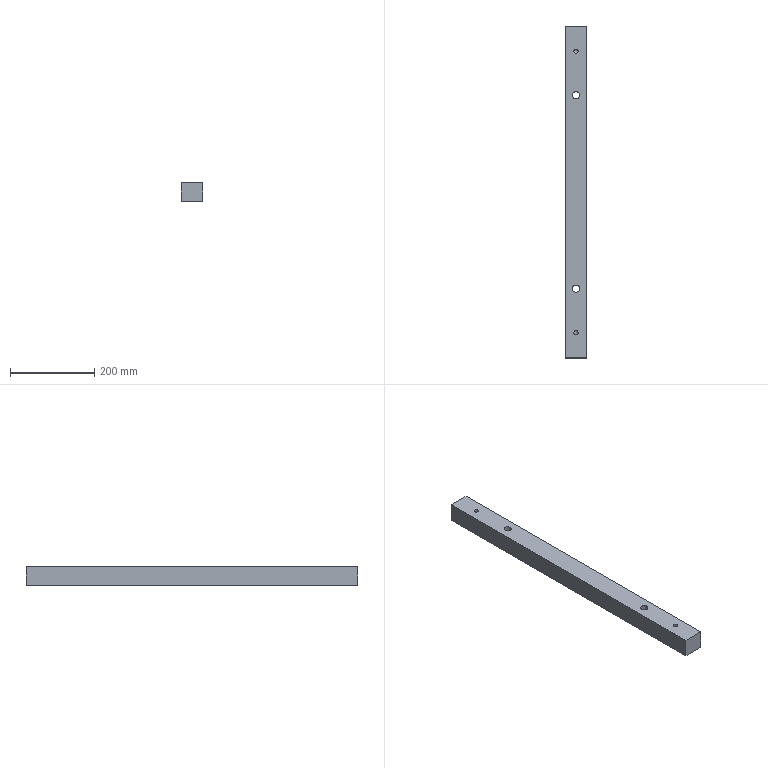Part | STEP file | 020_id2186_x_t | 1 solid | 12 faces | box 50 x 790 x 45 mm | volume 1752403 mm3 | plane 6 | cylinder 4 | cone 2 | commonest cylinder face diameters 10.3 x2 17 x2
STEP:
#1=CARTESIAN_POINT('',(0.,0.,0.));
#2=DIRECTION('',(0.,0.,1.));
#3=DIRECTION('',(1.,0.,0.));
#4=AXIS2_PLACEMENT_3D('',#1,#2,#3);
#5=CARTESIAN_POINT('',(168.35,335.,230.));
#6=VERTEX_POINT('',#5);
#7=CARTESIAN_POINT('',(173.5,335.,230.));
#8=DIRECTION('',(0.,0.,1.));
#9=DIRECTION('',(-1.,0.,0.));
#10=AXIS2_PLACEMENT_3D('',#7,#8,#9);
#11=CIRCLE('',#10,5.15);
#12=CARTESIAN_POINT('',(353.5,-140.,230.));
#13=DIRECTION('',(0.,0.,1.));
#14=DIRECTION('',(1.,0.,0.));
#15=AXIS2_PLACEMENT_3D('',#12,#13,#14);
#16=PLANE('',#15);
#17=CARTESIAN_POINT('',(-180.,475.));
#18=DIRECTION('',(-1.,0.));
#19=AXIS2_PLACEMENT_2D('',#17,#18);
#20=CIRCLE('',#19,5.15);
#21=(GEOMETRIC_REPRESENTATION_CONTEXT(2)PARAMETRIC_REPRESENTATION_CONTEXT()REPRESENTATION_CONTEXT('',''));
#22=DEFINITIONAL_REPRESENTATION('',(#20),#21);
#23=PCURVE('',#16,#22);
#24=CARTESIAN_POINT('',(173.5,335.,259.));
#25=DIRECTION('',(0.,0.,-1.));
#26=DIRECTION('',(-1.,0.,0.));
#27=AXIS2_PLACEMENT_3D('',#24,#25,#26);
#28=CYLINDRICAL_SURFACE('',#27,5.15);
#29=CARTESIAN_POINT('',(6.283,29.));
#30=DIRECTION('',(-1.,0.));
#31=VECTOR('',#30,1.);
#32=LINE('',#29,#31);
#33=(GEOMETRIC_REPRESENTATION_CONTEXT(2)PARAMETRIC_REPRESENTATION_CONTEXT()REPRESENTATION_CONTEXT('',''));
#34=DEFINITIONAL_REPRESENTATION('',(#32),#33);
#35=PCURVE('',#28,#34);
#36=SURFACE_CURVE('',#11,(#23,#35),.PCURVE_S1.);
#37=EDGE_CURVE('',#6,#6,#36,.T.);
#38=ORIENTED_EDGE('',*,*,#37,.F.);
#39=EDGE_LOOP('',(#38));
#40=FACE_BOUND('',#39,.T.);
#41=CARTESIAN_POINT('',(182.,230.,230.));
#42=VERTEX_POINT('',#41);
#43=CARTESIAN_POINT('',(173.5,230.,230.));
#44=DIRECTION('',(0.,0.,-1.));
#45=DIRECTION('',(1.,0.,0.));
#46=AXIS2_PLACEMENT_3D('',#43,#44,#45);
#47=CIRCLE('',#46,8.5);
#48=CARTESIAN_POINT('',(-171.5,370.));
#49=CARTESIAN_POINT('',(-171.5,355.278));
#50=CARTESIAN_POINT('',(-184.25,362.639));
#51=CARTESIAN_POINT('',(-197.,370.));
#52=CARTESIAN_POINT('',(-184.25,377.361));
#53=CARTESIAN_POINT('',(-171.5,384.722));
#54=CARTESIAN_POINT('',(-171.5,370.));
#55=(BOUNDED_CURVE()B_SPLINE_CURVE(2,(#48,#49,#50,#51,#52,#53,#54),.UNSPECIFIED.,.T.,.F.)B_SPLINE_CURVE_WITH_KNOTS((1,2,2,2,2,1),(-2.094,0.,2.094,4.189,6.283,8.378),.UNSPECIFIED.)CURVE()GEOMETRIC_REPRESENTATION_ITEM()RATIONAL_B_SPLINE_CURVE((1.,0.5,1.,0.5,1.,0.5,1.))REPRESENTATION_ITEM(''));
#56=(GEOMETRIC_REPRESENTATION_CONTEXT(2)PARAMETRIC_REPRESENTATION_CONTEXT()REPRESENTATION_CONTEXT('',''));
#57=DEFINITIONAL_REPRESENTATION('',(#55),#56);
#58=PCURVE('',#16,#57);
#59=CARTESIAN_POINT('',(173.5,230.,150.));
#60=DIRECTION('',(0.,0.,1.));
#61=DIRECTION('',(1.,0.,0.));
#62=AXIS2_PLACEMENT_3D('',#59,#60,#61);
#63=CYLINDRICAL_SURFACE('',#62,8.5);
#64=CARTESIAN_POINT('',(6.283,80.));
#65=DIRECTION('',(-1.,0.));
#66=VECTOR('',#65,1.);
#67=LINE('',#64,#66);
#68=(GEOMETRIC_REPRESENTATION_CONTEXT(2)PARAMETRIC_REPRESENTATION_CONTEXT()REPRESENTATION_CONTEXT('',''));
#69=DEFINITIONAL_REPRESENTATION('',(#67),#68);
#70=PCURVE('',#63,#69);
#71=SURFACE_CURVE('',#47,(#58,#70),.PCURVE_S1.);
#72=EDGE_CURVE('',#42,#42,#71,.T.);
#73=ORIENTED_EDGE('',*,*,#72,.T.);
#74=EDGE_LOOP('',(#73));
#75=FACE_BOUND('',#74,.T.);
#76=CARTESIAN_POINT('',(182.,-230.,230.));
#77=VERTEX_POINT('',#76);
#78=CARTESIAN_POINT('',(173.5,-230.,230.));
#79=DIRECTION('',(0.,0.,1.));
#80=DIRECTION('',(1.,0.,0.));
#81=AXIS2_PLACEMENT_3D('',#78,#79,#80);
#82=CIRCLE('',#81,8.5);
#83=CARTESIAN_POINT('',(-180.,-90.));
#84=DIRECTION('',(1.,0.));
#85=AXIS2_PLACEMENT_2D('',#83,#84);
#86=CIRCLE('',#85,8.5);
#87=(GEOMETRIC_REPRESENTATION_CONTEXT(2)PARAMETRIC_REPRESENTATION_CONTEXT()REPRESENTATION_CONTEXT('',''));
#88=DEFINITIONAL_REPRESENTATION('',(#86),#87);
#89=PCURVE('',#16,#88);
#90=CARTESIAN_POINT('',(173.5,-230.,150.));
#91=DIRECTION('',(0.,0.,1.));
#92=DIRECTION('',(1.,0.,0.));
#93=AXIS2_PLACEMENT_3D('',#90,#91,#92);
#94=CYLINDRICAL_SURFACE('',#93,8.5);
#95=CARTESIAN_POINT('',(0.,80.));
#96=DIRECTION('',(1.,0.));
#97=VECTOR('',#96,1.);
#98=LINE('',#95,#97);
#99=(GEOMETRIC_REPRESENTATION_CONTEXT(2)PARAMETRIC_REPRESENTATION_CONTEXT()REPRESENTATION_CONTEXT('',''));
#100=DEFINITIONAL_REPRESENTATION('',(#98),#99);
#101=PCURVE('',#94,#100);
#102=SURFACE_CURVE('',#82,(#89,#101),.PCURVE_S1.);
#103=EDGE_CURVE('',#77,#77,#102,.T.);
#104=ORIENTED_EDGE('',*,*,#103,.F.);
#105=EDGE_LOOP('',(#104));
#106=FACE_BOUND('',#105,.T.);
#107=CARTESIAN_POINT('',(198.5,395.,230.));
#108=VERTEX_POINT('',#107);
#109=CARTESIAN_POINT('',(148.5,395.,230.));
#110=VERTEX_POINT('',#109);
#111=CARTESIAN_POINT('',(353.5,395.,230.));
#112=DIRECTION('',(-1.,0.,0.));
#113=VECTOR('',#112,1.);
#114=LINE('',#111,#113);
#115=CARTESIAN_POINT('',(0.,535.));
#116=DIRECTION('',(-1.,0.));
#117=VECTOR('',#116,1.);
#118=LINE('',#115,#117);
#119=(GEOMETRIC_REPRESENTATION_CONTEXT(2)PARAMETRIC_REPRESENTATION_CONTEXT()REPRESENTATION_CONTEXT('',''));
#120=DEFINITIONAL_REPRESENTATION('',(#118),#119);
#121=PCURVE('',#16,#120);
#122=CARTESIAN_POINT('',(-566.5,395.,-116.5));
#123=DIRECTION('',(0.,1.,0.));
#124=DIRECTION('',(0.,0.,-1.));
#125=AXIS2_PLACEMENT_3D('',#122,#123,#124);
#126=PLANE('',#125);
#127=CARTESIAN_POINT('',(-346.5,-920.));
#128=DIRECTION('',(0.,1.));
#129=VECTOR('',#128,1.);
#130=LINE('',#127,#129);
#131=(GEOMETRIC_REPRESENTATION_CONTEXT(2)PARAMETRIC_REPRESENTATION_CONTEXT()REPRESENTATION_CONTEXT('',''));
#132=DEFINITIONAL_REPRESENTATION('',(#130),#131);
#133=PCURVE('',#126,#132);
#134=SURFACE_CURVE('',#114,(#121,#133),.PCURVE_S1.);
#135=EDGE_CURVE('',#108,#110,#134,.T.);
#136=ORIENTED_EDGE('',*,*,#135,.T.);
#137=CARTESIAN_POINT('',(148.5,-395.,230.));
#138=VERTEX_POINT('',#137);
#139=CARTESIAN_POINT('',(148.5,-350.,230.));
#140=DIRECTION('',(0.,-1.,0.));
#141=VECTOR('',#140,1.);
#142=LINE('',#139,#141);
#143=CARTESIAN_POINT('',(-205.,-210.));
#144=DIRECTION('',(0.,-1.));
#145=VECTOR('',#144,1.);
#146=LINE('',#143,#145);
#147=(GEOMETRIC_REPRESENTATION_CONTEXT(2)PARAMETRIC_REPRESENTATION_CONTEXT()REPRESENTATION_CONTEXT('',''));
#148=DEFINITIONAL_REPRESENTATION('',(#146),#147);
#149=PCURVE('',#16,#148);
#150=CARTESIAN_POINT('',(148.5,-350.,428.5));
#151=DIRECTION('',(-1.,0.,0.));
#152=DIRECTION('',(0.,0.,-1.));
#153=AXIS2_PLACEMENT_3D('',#150,#151,#152);
#154=PLANE('',#153);
#155=CARTESIAN_POINT('',(198.5,0.));
#156=DIRECTION('',(0.,1.));
#157=VECTOR('',#156,1.);
#158=LINE('',#155,#157);
#159=(GEOMETRIC_REPRESENTATION_CONTEXT(2)PARAMETRIC_REPRESENTATION_CONTEXT()REPRESENTATION_CONTEXT('',''));
#160=DEFINITIONAL_REPRESENTATION('',(#158),#159);
#161=PCURVE('',#154,#160);
#162=SURFACE_CURVE('',#142,(#149,#161),.PCURVE_S1.);
#163=EDGE_CURVE('',#110,#138,#162,.T.);
#164=ORIENTED_EDGE('',*,*,#163,.T.);
#165=CARTESIAN_POINT('',(198.5,-395.,230.));
#166=VERTEX_POINT('',#165);
#167=CARTESIAN_POINT('',(353.5,-395.,230.));
#168=DIRECTION('',(-1.,0.,0.));
#169=VECTOR('',#168,1.);
#170=LINE('',#167,#169);
#171=CARTESIAN_POINT('',(0.,-255.));
#172=DIRECTION('',(-1.,0.));
#173=VECTOR('',#172,1.);
#174=LINE('',#171,#173);
#175=(GEOMETRIC_REPRESENTATION_CONTEXT(2)PARAMETRIC_REPRESENTATION_CONTEXT()REPRESENTATION_CONTEXT('',''));
#176=DEFINITIONAL_REPRESENTATION('',(#174),#175);
#177=PCURVE('',#16,#176);
#178=CARTESIAN_POINT('',(-566.5,-395.,-116.5));
#179=DIRECTION('',(0.,-1.,0.));
#180=DIRECTION('',(0.,0.,1.));
#181=AXIS2_PLACEMENT_3D('',#178,#179,#180);
#182=PLANE('',#181);
#183=CARTESIAN_POINT('',(346.5,-920.));
#184=DIRECTION('',(0.,1.));
#185=VECTOR('',#184,1.);
#186=LINE('',#183,#185);
#187=(GEOMETRIC_REPRESENTATION_CONTEXT(2)PARAMETRIC_REPRESENTATION_CONTEXT()REPRESENTATION_CONTEXT('',''));
#188=DEFINITIONAL_REPRESENTATION('',(#186),#187);
#189=PCURVE('',#182,#188);
#190=SURFACE_CURVE('',#170,(#177,#189),.PCURVE_S1.);
#191=EDGE_CURVE('',#166,#138,#190,.T.);
#192=ORIENTED_EDGE('',*,*,#191,.F.);
#193=CARTESIAN_POINT('',(198.5,-350.,230.));
#194=DIRECTION('',(0.,1.,0.));
#195=VECTOR('',#194,1.);
#196=LINE('',#193,#195);
#197=CARTESIAN_POINT('',(-155.,-210.));
#198=DIRECTION('',(0.,1.));
#199=VECTOR('',#198,1.);
#200=LINE('',#197,#199);
#201=(GEOMETRIC_REPRESENTATION_CONTEXT(2)PARAMETRIC_REPRESENTATION_CONTEXT()REPRESENTATION_CONTEXT('',''));
#202=DEFINITIONAL_REPRESENTATION('',(#200),#201);
#203=PCURVE('',#16,#202);
#204=CARTESIAN_POINT('',(198.5,-350.,428.5));
#205=DIRECTION('',(-1.,0.,0.));
#206=DIRECTION('',(0.,0.,-1.));
#207=AXIS2_PLACEMENT_3D('',#204,#205,#206);
#208=PLANE('',#207);
#209=CARTESIAN_POINT('',(198.5,0.));
#210=DIRECTION('',(0.,-1.));
#211=VECTOR('',#210,1.);
#212=LINE('',#209,#211);
#213=(GEOMETRIC_REPRESENTATION_CONTEXT(2)PARAMETRIC_REPRESENTATION_CONTEXT()REPRESENTATION_CONTEXT('',''));
#214=DEFINITIONAL_REPRESENTATION('',(#212),#213);
#215=PCURVE('',#208,#214);
#216=SURFACE_CURVE('',#196,(#203,#215),.PCURVE_S1.);
#217=EDGE_CURVE('',#166,#108,#216,.T.);
#218=ORIENTED_EDGE('',*,*,#217,.T.);
#219=EDGE_LOOP('',(#136,#164,#192,#218));
#220=FACE_BOUND('',#219,.T.);
#221=CARTESIAN_POINT('',(168.35,-335.,230.));
#222=VERTEX_POINT('',#221);
#223=CARTESIAN_POINT('',(173.5,-335.,230.));
#224=DIRECTION('',(0.,0.,-1.));
#225=DIRECTION('',(-1.,0.,0.));
#226=AXIS2_PLACEMENT_3D('',#223,#224,#225);
#227=CIRCLE('',#226,5.15);
#228=CARTESIAN_POINT('',(-185.15,-195.));
#229=CARTESIAN_POINT('',(-185.15,-186.08));
#230=CARTESIAN_POINT('',(-177.425,-190.54));
#231=CARTESIAN_POINT('',(-169.7,-195.));
#232=CARTESIAN_POINT('',(-177.425,-199.46));
#233=CARTESIAN_POINT('',(-185.15,-203.92));
#234=CARTESIAN_POINT('',(-185.15,-195.));
#235=(BOUNDED_CURVE()B_SPLINE_CURVE(2,(#228,#229,#230,#231,#232,#233,#234),.UNSPECIFIED.,.T.,.F.)B_SPLINE_CURVE_WITH_KNOTS((1,2,2,2,2,1),(-2.094,0.,2.094,4.189,6.283,8.378),.UNSPECIFIED.)CURVE()GEOMETRIC_REPRESENTATION_ITEM()RATIONAL_B_SPLINE_CURVE((1.,0.5,1.,0.5,1.,0.5,1.))REPRESENTATION_ITEM(''));
#236=(GEOMETRIC_REPRESENTATION_CONTEXT(2)PARAMETRIC_REPRESENTATION_CONTEXT()REPRESENTATION_CONTEXT('',''));
#237=DEFINITIONAL_REPRESENTATION('',(#235),#236);
#238=PCURVE('',#16,#237);
#239=CARTESIAN_POINT('',(173.5,-335.,259.));
#240=DIRECTION('',(0.,0.,-1.));
#241=DIRECTION('',(-1.,0.,0.));
#242=AXIS2_PLACEMENT_3D('',#239,#240,#241);
#243=CYLINDRICAL_SURFACE('',#242,5.15);
#244=CARTESIAN_POINT('',(0.,29.));
#245=DIRECTION('',(1.,0.));
#246=VECTOR('',#245,1.);
#247=LINE('',#244,#246);
#248=(GEOMETRIC_REPRESENTATION_CONTEXT(2)PARAMETRIC_REPRESENTATION_CONTEXT()REPRESENTATION_CONTEXT('',''));
#249=DEFINITIONAL_REPRESENTATION('',(#247),#248);
#250=PCURVE('',#243,#249);
#251=SURFACE_CURVE('',#227,(#238,#250),.PCURVE_S1.);
#252=EDGE_CURVE('',#222,#222,#251,.T.);
#253=ORIENTED_EDGE('',*,*,#252,.T.);
#254=EDGE_LOOP('',(#253));
#255=FACE_BOUND('',#254,.T.);
#256=ADVANCED_FACE('',(#40,#75,#106,#220,#255),#16,.T.);
#257=CARTESIAN_POINT('',(198.5,-395.,185.));
#258=VERTEX_POINT('',#257);
#259=CARTESIAN_POINT('',(148.5,-395.,185.));
#260=VERTEX_POINT('',#259);
#261=CARTESIAN_POINT('',(-566.5,-395.,185.));
#262=DIRECTION('',(-1.,0.,0.));
#263=VECTOR('',#262,1.);
#264=LINE('',#261,#263);
#265=CARTESIAN_POINT('',(148.5,-350.,185.));
#266=DIRECTION('',(0.,0.,1.));
#267=DIRECTION('',(0.,-1.,0.));
#268=AXIS2_PLACEMENT_3D('',#265,#266,#267);
#269=PLANE('',#268);
#270=CARTESIAN_POINT('',(45.,-715.));
#271=DIRECTION('',(0.,-1.));
#272=VECTOR('',#271,1.);
#273=LINE('',#270,#272);
#274=(GEOMETRIC_REPRESENTATION_CONTEXT(2)PARAMETRIC_REPRESENTATION_CONTEXT()REPRESENTATION_CONTEXT('',''));
#275=DEFINITIONAL_REPRESENTATION('',(#273),#274);
#276=PCURVE('',#269,#275);
#277=CARTESIAN_POINT('',(301.5,0.));
#278=DIRECTION('',(0.,1.));
#279=VECTOR('',#278,1.);
#280=LINE('',#277,#279);
#281=(GEOMETRIC_REPRESENTATION_CONTEXT(2)PARAMETRIC_REPRESENTATION_CONTEXT()REPRESENTATION_CONTEXT('',''));
#282=DEFINITIONAL_REPRESENTATION('',(#280),#281);
#283=PCURVE('',#182,#282);
#284=SURFACE_CURVE('',#264,(#276,#283),.PCURVE_S1.);
#285=EDGE_CURVE('',#258,#260,#284,.T.);
#286=ORIENTED_EDGE('',*,*,#285,.T.);
#287=CARTESIAN_POINT('',(148.5,395.,185.));
#288=VERTEX_POINT('',#287);
#289=CARTESIAN_POINT('',(148.5,-350.,185.));
#290=DIRECTION('',(0.,1.,0.));
#291=VECTOR('',#290,1.);
#292=LINE('',#289,#291);
#293=CARTESIAN_POINT('',(0.,0.));
#294=DIRECTION('',(-1.,0.));
#295=VECTOR('',#294,1.);
#296=LINE('',#293,#295);
#297=(GEOMETRIC_REPRESENTATION_CONTEXT(2)PARAMETRIC_REPRESENTATION_CONTEXT()REPRESENTATION_CONTEXT('',''));
#298=DEFINITIONAL_REPRESENTATION('',(#296),#297);
#299=PCURVE('',#269,#298);
#300=CARTESIAN_POINT('',(243.5,0.));
#301=DIRECTION('',(0.,-1.));
#302=VECTOR('',#301,1.);
#303=LINE('',#300,#302);
#304=(GEOMETRIC_REPRESENTATION_CONTEXT(2)PARAMETRIC_REPRESENTATION_CONTEXT()REPRESENTATION_CONTEXT('',''));
#305=DEFINITIONAL_REPRESENTATION('',(#303),#304);
#306=PCURVE('',#154,#305);
#307=SURFACE_CURVE('',#292,(#299,#306),.PCURVE_S1.);
#308=EDGE_CURVE('',#260,#288,#307,.T.);
#309=ORIENTED_EDGE('',*,*,#308,.T.);
#310=CARTESIAN_POINT('',(198.5,395.,185.));
#311=VERTEX_POINT('',#310);
#312=CARTESIAN_POINT('',(148.5,395.,185.));
#313=DIRECTION('',(-1.,0.,0.));
#314=VECTOR('',#313,1.);
#315=LINE('',#312,#314);
#316=CARTESIAN_POINT('',(-745.,0.));
#317=DIRECTION('',(0.,-1.));
#318=VECTOR('',#317,1.);
#319=LINE('',#316,#318);
#320=(GEOMETRIC_REPRESENTATION_CONTEXT(2)PARAMETRIC_REPRESENTATION_CONTEXT()REPRESENTATION_CONTEXT('',''));
#321=DEFINITIONAL_REPRESENTATION('',(#319),#320);
#322=PCURVE('',#269,#321);
#323=CARTESIAN_POINT('',(-301.5,-715.));
#324=DIRECTION('',(0.,1.));
#325=VECTOR('',#324,1.);
#326=LINE('',#323,#325);
#327=(GEOMETRIC_REPRESENTATION_CONTEXT(2)PARAMETRIC_REPRESENTATION_CONTEXT()REPRESENTATION_CONTEXT('',''));
#328=DEFINITIONAL_REPRESENTATION('',(#326),#327);
#329=PCURVE('',#126,#328);
#330=SURFACE_CURVE('',#315,(#322,#329),.PCURVE_S1.);
#331=EDGE_CURVE('',#311,#288,#330,.T.);
#332=ORIENTED_EDGE('',*,*,#331,.F.);
#333=CARTESIAN_POINT('',(198.5,-350.,185.));
#334=DIRECTION('',(0.,1.,0.));
#335=VECTOR('',#334,1.);
#336=LINE('',#333,#335);
#337=CARTESIAN_POINT('',(0.,50.));
#338=DIRECTION('',(-1.,0.));
#339=VECTOR('',#338,1.);
#340=LINE('',#337,#339);
#341=(GEOMETRIC_REPRESENTATION_CONTEXT(2)PARAMETRIC_REPRESENTATION_CONTEXT()REPRESENTATION_CONTEXT('',''));
#342=DEFINITIONAL_REPRESENTATION('',(#340),#341);
#343=PCURVE('',#269,#342);
#344=CARTESIAN_POINT('',(243.5,0.));
#345=DIRECTION('',(0.,-1.));
#346=VECTOR('',#345,1.);
#347=LINE('',#344,#346);
#348=(GEOMETRIC_REPRESENTATION_CONTEXT(2)PARAMETRIC_REPRESENTATION_CONTEXT()REPRESENTATION_CONTEXT('',''));
#349=DEFINITIONAL_REPRESENTATION('',(#347),#348);
#350=PCURVE('',#208,#349);
#351=SURFACE_CURVE('',#336,(#343,#350),.PCURVE_S1.);
#352=EDGE_CURVE('',#258,#311,#351,.T.);
#353=ORIENTED_EDGE('',*,*,#352,.F.);
#354=EDGE_LOOP('',(#286,#309,#332,#353));
#355=FACE_BOUND('',#354,.T.);
#356=CARTESIAN_POINT('',(182.,-230.,185.));
#357=VERTEX_POINT('',#356);
#358=CARTESIAN_POINT('',(173.5,-230.,185.));
#359=DIRECTION('',(0.,0.,1.));
#360=DIRECTION('',(1.,0.,0.));
#361=AXIS2_PLACEMENT_3D('',#358,#359,#360);
#362=CIRCLE('',#361,8.5);
#363=CARTESIAN_POINT('',(-120.,25.));
#364=DIRECTION('',(0.,1.));
#365=AXIS2_PLACEMENT_2D('',#363,#364);
#366=CIRCLE('',#365,8.5);
#367=(GEOMETRIC_REPRESENTATION_CONTEXT(2)PARAMETRIC_REPRESENTATION_CONTEXT()REPRESENTATION_CONTEXT('',''));
#368=DEFINITIONAL_REPRESENTATION('',(#366),#367);
#369=PCURVE('',#269,#368);
#370=CARTESIAN_POINT('',(0.,35.));
#371=DIRECTION('',(1.,0.));
#372=VECTOR('',#371,1.);
#373=LINE('',#370,#372);
#374=(GEOMETRIC_REPRESENTATION_CONTEXT(2)PARAMETRIC_REPRESENTATION_CONTEXT()REPRESENTATION_CONTEXT('',''));
#375=DEFINITIONAL_REPRESENTATION('',(#373),#374);
#376=PCURVE('',#94,#375);
#377=SURFACE_CURVE('',#362,(#369,#376),.PCURVE_S1.);
#378=EDGE_CURVE('',#357,#357,#377,.T.);
#379=ORIENTED_EDGE('',*,*,#378,.T.);
#380=EDGE_LOOP('',(#379));
#381=FACE_BOUND('',#380,.T.);
#382=CARTESIAN_POINT('',(182.,230.,185.));
#383=VERTEX_POINT('',#382);
#384=CARTESIAN_POINT('',(173.5,230.,185.));
#385=DIRECTION('',(0.,0.,-1.));
#386=DIRECTION('',(1.,0.,0.));
#387=AXIS2_PLACEMENT_3D('',#384,#385,#386);
#388=CIRCLE('',#387,8.5);
#389=CARTESIAN_POINT('',(-580.,33.5));
#390=CARTESIAN_POINT('',(-565.278,33.5));
#391=CARTESIAN_POINT('',(-572.639,20.75));
#392=CARTESIAN_POINT('',(-580.,8.));
#393=CARTESIAN_POINT('',(-587.361,20.75));
#394=CARTESIAN_POINT('',(-594.722,33.5));
#395=CARTESIAN_POINT('',(-580.,33.5));
#396=(BOUNDED_CURVE()B_SPLINE_CURVE(2,(#389,#390,#391,#392,#393,#394,#395),.UNSPECIFIED.,.T.,.F.)B_SPLINE_CURVE_WITH_KNOTS((1,2,2,2,2,1),(-2.094,0.,2.094,4.189,6.283,8.378),.UNSPECIFIED.)CURVE()GEOMETRIC_REPRESENTATION_ITEM()RATIONAL_B_SPLINE_CURVE((1.,0.5,1.,0.5,1.,0.5,1.))REPRESENTATION_ITEM(''));
#397=(GEOMETRIC_REPRESENTATION_CONTEXT(2)PARAMETRIC_REPRESENTATION_CONTEXT()REPRESENTATION_CONTEXT('',''));
#398=DEFINITIONAL_REPRESENTATION('',(#396),#397);
#399=PCURVE('',#269,#398);
#400=CARTESIAN_POINT('',(6.283,35.));
#401=DIRECTION('',(-1.,0.));
#402=VECTOR('',#401,1.);
#403=LINE('',#400,#402);
#404=(GEOMETRIC_REPRESENTATION_CONTEXT(2)PARAMETRIC_REPRESENTATION_CONTEXT()REPRESENTATION_CONTEXT('',''));
#405=DEFINITIONAL_REPRESENTATION('',(#403),#404);
#406=PCURVE('',#63,#405);
#407=SURFACE_CURVE('',#388,(#399,#406),.PCURVE_S1.);
#408=EDGE_CURVE('',#383,#383,#407,.T.);
#409=ORIENTED_EDGE('',*,*,#408,.F.);
#410=EDGE_LOOP('',(#409));
#411=FACE_BOUND('',#410,.T.);
#412=ADVANCED_FACE('',(#355,#381,#411),#269,.F.);
#413=ORIENTED_EDGE('',*,*,#217,.F.);
#414=CARTESIAN_POINT('',(198.5,-395.,428.5));
#415=DIRECTION('',(0.,0.,-1.));
#416=VECTOR('',#415,1.);
#417=LINE('',#414,#416);
#418=CARTESIAN_POINT('',(0.,45.));
#419=DIRECTION('',(1.,0.));
#420=VECTOR('',#419,1.);
#421=LINE('',#418,#420);
#422=(GEOMETRIC_REPRESENTATION_CONTEXT(2)PARAMETRIC_REPRESENTATION_CONTEXT()REPRESENTATION_CONTEXT('',''));
#423=DEFINITIONAL_REPRESENTATION('',(#421),#422);
#424=PCURVE('',#208,#423);
#425=CARTESIAN_POINT('',(545.,-765.));
#426=DIRECTION('',(-1.,0.));
#427=VECTOR('',#426,1.);
#428=LINE('',#425,#427);
#429=(GEOMETRIC_REPRESENTATION_CONTEXT(2)PARAMETRIC_REPRESENTATION_CONTEXT()REPRESENTATION_CONTEXT('',''));
#430=DEFINITIONAL_REPRESENTATION('',(#428),#429);
#431=PCURVE('',#182,#430);
#432=SURFACE_CURVE('',#417,(#424,#431),.PCURVE_S1.);
#433=EDGE_CURVE('',#166,#258,#432,.T.);
#434=ORIENTED_EDGE('',*,*,#433,.T.);
#435=ORIENTED_EDGE('',*,*,#352,.T.);
#436=CARTESIAN_POINT('',(198.5,395.,-116.5));
#437=DIRECTION('',(0.,0.,1.));
#438=VECTOR('',#437,1.);
#439=LINE('',#436,#438);
#440=CARTESIAN_POINT('',(545.,-745.));
#441=DIRECTION('',(-1.,0.));
#442=VECTOR('',#441,1.);
#443=LINE('',#440,#442);
#444=(GEOMETRIC_REPRESENTATION_CONTEXT(2)PARAMETRIC_REPRESENTATION_CONTEXT()REPRESENTATION_CONTEXT('',''));
#445=DEFINITIONAL_REPRESENTATION('',(#443),#444);
#446=PCURVE('',#208,#445);
#447=CARTESIAN_POINT('',(0.,-765.));
#448=DIRECTION('',(-1.,0.));
#449=VECTOR('',#448,1.);
#450=LINE('',#447,#449);
#451=(GEOMETRIC_REPRESENTATION_CONTEXT(2)PARAMETRIC_REPRESENTATION_CONTEXT()REPRESENTATION_CONTEXT('',''));
#452=DEFINITIONAL_REPRESENTATION('',(#450),#451);
#453=PCURVE('',#126,#452);
#454=SURFACE_CURVE('',#439,(#446,#453),.PCURVE_S1.);
#455=EDGE_CURVE('',#311,#108,#454,.T.);
#456=ORIENTED_EDGE('',*,*,#455,.T.);
#457=EDGE_LOOP('',(#413,#434,#435,#456));
#458=FACE_BOUND('',#457,.T.);
#459=ADVANCED_FACE('',(#458),#208,.F.);
#460=ORIENTED_EDGE('',*,*,#191,.T.);
#461=CARTESIAN_POINT('',(148.5,-395.,428.5));
#462=DIRECTION('',(0.,0.,-1.));
#463=VECTOR('',#462,1.);
#464=LINE('',#461,#463);
#465=CARTESIAN_POINT('',(545.,-715.));
#466=DIRECTION('',(-1.,0.));
#467=VECTOR('',#466,1.);
#468=LINE('',#465,#467);
#469=(GEOMETRIC_REPRESENTATION_CONTEXT(2)PARAMETRIC_REPRESENTATION_CONTEXT()REPRESENTATION_CONTEXT('',''));
#470=DEFINITIONAL_REPRESENTATION('',(#468),#469);
#471=PCURVE('',#182,#470);
#472=CARTESIAN_POINT('',(0.,45.));
#473=DIRECTION('',(1.,0.));
#474=VECTOR('',#473,1.);
#475=LINE('',#472,#474);
#476=(GEOMETRIC_REPRESENTATION_CONTEXT(2)PARAMETRIC_REPRESENTATION_CONTEXT()REPRESENTATION_CONTEXT('',''));
#477=DEFINITIONAL_REPRESENTATION('',(#475),#476);
#478=PCURVE('',#154,#477);
#479=SURFACE_CURVE('',#464,(#471,#478),.PCURVE_S1.);
#480=EDGE_CURVE('',#138,#260,#479,.T.);
#481=ORIENTED_EDGE('',*,*,#480,.T.);
#482=ORIENTED_EDGE('',*,*,#285,.F.);
#483=ORIENTED_EDGE('',*,*,#433,.F.);
#484=EDGE_LOOP('',(#460,#481,#482,#483));
#485=FACE_BOUND('',#484,.T.);
#486=ADVANCED_FACE('',(#485),#182,.T.);
#487=CARTESIAN_POINT('',(148.5,395.,-116.5));
#488=DIRECTION('',(0.,0.,1.));
#489=VECTOR('',#488,1.);
#490=LINE('',#487,#489);
#491=CARTESIAN_POINT('',(545.,-745.));
#492=DIRECTION('',(-1.,0.));
#493=VECTOR('',#492,1.);
#494=LINE('',#491,#493);
#495=(GEOMETRIC_REPRESENTATION_CONTEXT(2)PARAMETRIC_REPRESENTATION_CONTEXT()REPRESENTATION_CONTEXT('',''));
#496=DEFINITIONAL_REPRESENTATION('',(#494),#495);
#497=PCURVE('',#154,#496);
#498=CARTESIAN_POINT('',(0.,-715.));
#499=DIRECTION('',(-1.,0.));
#500=VECTOR('',#499,1.);
#501=LINE('',#498,#500);
#502=(GEOMETRIC_REPRESENTATION_CONTEXT(2)PARAMETRIC_REPRESENTATION_CONTEXT()REPRESENTATION_CONTEXT('',''));
#503=DEFINITIONAL_REPRESENTATION('',(#501),#502);
#504=PCURVE('',#126,#503);
#505=SURFACE_CURVE('',#490,(#497,#504),.PCURVE_S1.);
#506=EDGE_CURVE('',#288,#110,#505,.T.);
#507=ORIENTED_EDGE('',*,*,#506,.F.);
#508=ORIENTED_EDGE('',*,*,#308,.F.);
#509=ORIENTED_EDGE('',*,*,#480,.F.);
#510=ORIENTED_EDGE('',*,*,#163,.F.);
#511=EDGE_LOOP('',(#507,#508,#509,#510));
#512=FACE_BOUND('',#511,.T.);
#513=ADVANCED_FACE('',(#512),#154,.T.);
#514=ORIENTED_EDGE('',*,*,#455,.F.);
#515=ORIENTED_EDGE('',*,*,#331,.T.);
#516=ORIENTED_EDGE('',*,*,#506,.T.);
#517=ORIENTED_EDGE('',*,*,#135,.F.);
#518=EDGE_LOOP('',(#514,#515,#516,#517));
#519=FACE_BOUND('',#518,.T.);
#520=ADVANCED_FACE('',(#519),#126,.T.);
#521=ORIENTED_EDGE('',*,*,#103,.F.);
#522=CARTESIAN_POINT('',(182.,-230.,185.));
#523=CARTESIAN_POINT('',(182.,-230.,230.));
#524=B_SPLINE_CURVE_WITH_KNOTS('',1,(#522,#523),.UNSPECIFIED.,.F.,.F.,(2,2),(35.,80.),.PIECEWISE_BEZIER_KNOTS.);
#525=CARTESIAN_POINT('',(0.,0.));
#526=DIRECTION('',(0.,1.));
#527=VECTOR('',#526,1.);
#528=LINE('',#525,#527);
#529=(GEOMETRIC_REPRESENTATION_CONTEXT(2)PARAMETRIC_REPRESENTATION_CONTEXT()REPRESENTATION_CONTEXT('',''));
#530=DEFINITIONAL_REPRESENTATION('',(#528),#529);
#531=PCURVE('',#94,#530);
#532=CARTESIAN_POINT('',(6.283,0.));
#533=DIRECTION('',(0.,1.));
#534=VECTOR('',#533,1.);
#535=LINE('',#532,#534);
#536=(GEOMETRIC_REPRESENTATION_CONTEXT(2)PARAMETRIC_REPRESENTATION_CONTEXT()REPRESENTATION_CONTEXT('',''));
#537=DEFINITIONAL_REPRESENTATION('',(#535),#536);
#538=PCURVE('',#94,#537);
#539=SEAM_CURVE('',#524,(#531,#538),.PCURVE_S1.);
#540=EDGE_CURVE('',#357,#77,#539,.T.);
#541=ORIENTED_EDGE('',*,*,#540,.F.);
#542=ORIENTED_EDGE('',*,*,#378,.T.);
#543=ORIENTED_EDGE('',*,*,#540,.T.);
#544=EDGE_LOOP('',(#521,#541,#542,#543));
#545=FACE_BOUND('',#544,.F.);
#546=ADVANCED_FACE('',(#545),#94,.F.);
#547=ORIENTED_EDGE('',*,*,#72,.T.);
#548=CARTESIAN_POINT('',(182.,230.,185.));
#549=CARTESIAN_POINT('',(182.,230.,230.));
#550=B_SPLINE_CURVE_WITH_KNOTS('',1,(#548,#549),.UNSPECIFIED.,.F.,.F.,(2,2),(35.,80.),.PIECEWISE_BEZIER_KNOTS.);
#551=CARTESIAN_POINT('',(0.,0.));
#552=DIRECTION('',(0.,1.));
#553=VECTOR('',#552,1.);
#554=LINE('',#551,#553);
#555=(GEOMETRIC_REPRESENTATION_CONTEXT(2)PARAMETRIC_REPRESENTATION_CONTEXT()REPRESENTATION_CONTEXT('',''));
#556=DEFINITIONAL_REPRESENTATION('',(#554),#555);
#557=PCURVE('',#63,#556);
#558=CARTESIAN_POINT('',(6.283,0.));
#559=DIRECTION('',(0.,1.));
#560=VECTOR('',#559,1.);
#561=LINE('',#558,#560);
#562=(GEOMETRIC_REPRESENTATION_CONTEXT(2)PARAMETRIC_REPRESENTATION_CONTEXT()REPRESENTATION_CONTEXT('',''));
#563=DEFINITIONAL_REPRESENTATION('',(#561),#562);
#564=PCURVE('',#63,#563);
#565=SEAM_CURVE('',#550,(#557,#564),.PCURVE_S1.);
#566=EDGE_CURVE('',#383,#42,#565,.T.);
#567=ORIENTED_EDGE('',*,*,#566,.F.);
#568=ORIENTED_EDGE('',*,*,#408,.F.);
#569=ORIENTED_EDGE('',*,*,#566,.T.);
#570=EDGE_LOOP('',(#547,#567,#568,#569));
#571=FACE_BOUND('',#570,.F.);
#572=ADVANCED_FACE('',(#571),#63,.F.);
#573=ORIENTED_EDGE('',*,*,#37,.F.);
#574=CARTESIAN_POINT('',(168.35,335.,202.973));
#575=VERTEX_POINT('',#574);
#576=CARTESIAN_POINT('',(168.35,335.,230.));
#577=CARTESIAN_POINT('',(168.35,335.,202.973));
#578=B_SPLINE_CURVE_WITH_KNOTS('',1,(#576,#577),.UNSPECIFIED.,.F.,.F.,(2,2),(29.,56.027),.PIECEWISE_BEZIER_KNOTS.);
#579=CARTESIAN_POINT('',(6.283,0.));
#580=DIRECTION('',(0.,1.));
#581=VECTOR('',#580,1.);
#582=LINE('',#579,#581);
#583=(GEOMETRIC_REPRESENTATION_CONTEXT(2)PARAMETRIC_REPRESENTATION_CONTEXT()REPRESENTATION_CONTEXT('',''));
#584=DEFINITIONAL_REPRESENTATION('',(#582),#583);
#585=PCURVE('',#28,#584);
#586=CARTESIAN_POINT('',(0.,0.));
#587=DIRECTION('',(0.,1.));
#588=VECTOR('',#587,1.);
#589=LINE('',#586,#588);
#590=(GEOMETRIC_REPRESENTATION_CONTEXT(2)PARAMETRIC_REPRESENTATION_CONTEXT()REPRESENTATION_CONTEXT('',''));
#591=DEFINITIONAL_REPRESENTATION('',(#589),#590);
#592=PCURVE('',#28,#591);
#593=SEAM_CURVE('',#578,(#585,#592),.PCURVE_S1.);
#594=EDGE_CURVE('',#6,#575,#593,.T.);
#595=ORIENTED_EDGE('',*,*,#594,.T.);
#596=CARTESIAN_POINT('',(178.65,335.,202.973));
#597=VERTEX_POINT('',#596);
#598=CARTESIAN_POINT('',(173.5,335.,202.973));
#599=DIRECTION('',(0.,0.,1.));
#600=DIRECTION('',(1.,0.,0.));
#601=AXIS2_PLACEMENT_3D('',#598,#599,#600);
#602=CIRCLE('',#601,5.15);
#603=CARTESIAN_POINT('',(9.425,56.027));
#604=DIRECTION('',(-1.,0.));
#605=VECTOR('',#604,1.);
#606=LINE('',#603,#605);
#607=(GEOMETRIC_REPRESENTATION_CONTEXT(2)PARAMETRIC_REPRESENTATION_CONTEXT()REPRESENTATION_CONTEXT('',''));
#608=DEFINITIONAL_REPRESENTATION('',(#606),#607);
#609=PCURVE('',#28,#608);
#610=CARTESIAN_POINT('',(173.5,335.,202.944));
#611=DIRECTION('',(0.,0.,1.));
#612=DIRECTION('',(1.,0.,0.));
#613=AXIS2_PLACEMENT_3D('',#610,#611,#612);
#614=CONICAL_SURFACE('',#613,5.1,1.047);
#615=CARTESIAN_POINT('',(0.,0.02887));
#616=DIRECTION('',(1.,0.));
#617=VECTOR('',#616,1.);
#618=LINE('',#615,#617);
#619=(GEOMETRIC_REPRESENTATION_CONTEXT(2)PARAMETRIC_REPRESENTATION_CONTEXT()REPRESENTATION_CONTEXT('',''));
#620=DEFINITIONAL_REPRESENTATION('',(#618),#619);
#621=PCURVE('',#614,#620);
#622=SURFACE_CURVE('',#602,(#609,#621),.PCURVE_S1.);
#623=EDGE_CURVE('',#575,#597,#622,.T.);
#624=ORIENTED_EDGE('',*,*,#623,.T.);
#625=CARTESIAN_POINT('',(173.5,335.,202.973));
#626=DIRECTION('',(0.,0.,1.));
#627=DIRECTION('',(1.,0.,0.));
#628=AXIS2_PLACEMENT_3D('',#625,#626,#627);
#629=CIRCLE('',#628,5.15);
#630=CARTESIAN_POINT('',(3.142,56.027));
#631=DIRECTION('',(-1.,0.));
#632=VECTOR('',#631,1.);
#633=LINE('',#630,#632);
#634=(GEOMETRIC_REPRESENTATION_CONTEXT(2)PARAMETRIC_REPRESENTATION_CONTEXT()REPRESENTATION_CONTEXT('',''));
#635=DEFINITIONAL_REPRESENTATION('',(#633),#634);
#636=PCURVE('',#28,#635);
#637=CARTESIAN_POINT('',(0.,0.02887));
#638=DIRECTION('',(1.,0.));
#639=VECTOR('',#638,1.);
#640=LINE('',#637,#639);
#641=(GEOMETRIC_REPRESENTATION_CONTEXT(2)PARAMETRIC_REPRESENTATION_CONTEXT()REPRESENTATION_CONTEXT('',''));
#642=DEFINITIONAL_REPRESENTATION('',(#640),#641);
#643=PCURVE('',#614,#642);
#644=SURFACE_CURVE('',#629,(#636,#643),.PCURVE_S1.);
#645=EDGE_CURVE('',#597,#575,#644,.T.);
#646=ORIENTED_EDGE('',*,*,#645,.T.);
#647=ORIENTED_EDGE('',*,*,#594,.F.);
#648=EDGE_LOOP('',(#573,#595,#624,#646,#647));
#649=FACE_BOUND('',#648,.F.);
#650=ADVANCED_FACE('',(#649),#28,.F.);
#651=CARTESIAN_POINT('',(173.5,335.,200.));
#652=VERTEX_POINT('',#651);
#653=CARTESIAN_POINT('',(173.5,335.,200.));
#654=CARTESIAN_POINT('',(178.65,335.,202.973));
#655=B_SPLINE_CURVE_WITH_KNOTS('',1,(#653,#654),.UNSPECIFIED.,.F.,.F.,(2,2),(-5.889,0.05774),.PIECEWISE_BEZIER_KNOTS.);
#656=CARTESIAN_POINT('',(6.283,0.));
#657=DIRECTION('',(0.,1.));
#658=VECTOR('',#657,1.);
#659=LINE('',#656,#658);
#660=(GEOMETRIC_REPRESENTATION_CONTEXT(2)PARAMETRIC_REPRESENTATION_CONTEXT()REPRESENTATION_CONTEXT('',''));
#661=DEFINITIONAL_REPRESENTATION('',(#659),#660);
#662=PCURVE('',#614,#661);
#663=CARTESIAN_POINT('',(0.,0.));
#664=DIRECTION('',(0.,1.));
#665=VECTOR('',#664,1.);
#666=LINE('',#663,#665);
#667=(GEOMETRIC_REPRESENTATION_CONTEXT(2)PARAMETRIC_REPRESENTATION_CONTEXT()REPRESENTATION_CONTEXT('',''));
#668=DEFINITIONAL_REPRESENTATION('',(#666),#667);
#669=PCURVE('',#614,#668);
#670=SEAM_CURVE('',#655,(#662,#669),.PCURVE_S1.);
#671=EDGE_CURVE('',#652,#597,#670,.T.);
#672=ORIENTED_EDGE('',*,*,#671,.T.);
#673=ORIENTED_EDGE('',*,*,#623,.F.);
#674=ORIENTED_EDGE('',*,*,#645,.F.);
#675=ORIENTED_EDGE('',*,*,#671,.F.);
#676=EDGE_LOOP('',(#672,#673,#674,#675));
#677=FACE_BOUND('',#676,.F.);
#678=ADVANCED_FACE('',(#677),#614,.F.);
#679=ORIENTED_EDGE('',*,*,#252,.T.);
#680=CARTESIAN_POINT('',(168.35,-335.,202.973));
#681=VERTEX_POINT('',#680);
#682=CARTESIAN_POINT('',(168.35,-335.,230.));
#683=CARTESIAN_POINT('',(168.35,-335.,202.973));
#684=B_SPLINE_CURVE_WITH_KNOTS('',1,(#682,#683),.UNSPECIFIED.,.F.,.F.,(2,2),(29.,56.027),.PIECEWISE_BEZIER_KNOTS.);
#685=CARTESIAN_POINT('',(6.283,0.));
#686=DIRECTION('',(0.,1.));
#687=VECTOR('',#686,1.);
#688=LINE('',#685,#687);
#689=(GEOMETRIC_REPRESENTATION_CONTEXT(2)PARAMETRIC_REPRESENTATION_CONTEXT()REPRESENTATION_CONTEXT('',''));
#690=DEFINITIONAL_REPRESENTATION('',(#688),#689);
#691=PCURVE('',#243,#690);
#692=CARTESIAN_POINT('',(0.,0.));
#693=DIRECTION('',(0.,1.));
#694=VECTOR('',#693,1.);
#695=LINE('',#692,#694);
#696=(GEOMETRIC_REPRESENTATION_CONTEXT(2)PARAMETRIC_REPRESENTATION_CONTEXT()REPRESENTATION_CONTEXT('',''));
#697=DEFINITIONAL_REPRESENTATION('',(#695),#696);
#698=PCURVE('',#243,#697);
#699=SEAM_CURVE('',#684,(#691,#698),.PCURVE_S1.);
#700=EDGE_CURVE('',#222,#681,#699,.T.);
#701=ORIENTED_EDGE('',*,*,#700,.T.);
#702=CARTESIAN_POINT('',(178.65,-335.,202.973));
#703=VERTEX_POINT('',#702);
#704=CARTESIAN_POINT('',(173.5,-335.,202.973));
#705=DIRECTION('',(0.,0.,-1.));
#706=DIRECTION('',(1.,0.,0.));
#707=AXIS2_PLACEMENT_3D('',#704,#705,#706);
#708=CIRCLE('',#707,5.15);
#709=CARTESIAN_POINT('',(3.142,56.027));
#710=DIRECTION('',(1.,0.));
#711=VECTOR('',#710,1.);
#712=LINE('',#709,#711);
#713=(GEOMETRIC_REPRESENTATION_CONTEXT(2)PARAMETRIC_REPRESENTATION_CONTEXT()REPRESENTATION_CONTEXT('',''));
#714=DEFINITIONAL_REPRESENTATION('',(#712),#713);
#715=PCURVE('',#243,#714);
#716=CARTESIAN_POINT('',(173.5,-335.,202.944));
#717=DIRECTION('',(0.,0.,1.));
#718=DIRECTION('',(1.,0.,0.));
#719=AXIS2_PLACEMENT_3D('',#716,#717,#718);
#720=CONICAL_SURFACE('',#719,5.1,1.047);
#721=CARTESIAN_POINT('',(6.283,0.02887));
#722=DIRECTION('',(-1.,0.));
#723=VECTOR('',#722,1.);
#724=LINE('',#721,#723);
#725=(GEOMETRIC_REPRESENTATION_CONTEXT(2)PARAMETRIC_REPRESENTATION_CONTEXT()REPRESENTATION_CONTEXT('',''));
#726=DEFINITIONAL_REPRESENTATION('',(#724),#725);
#727=PCURVE('',#720,#726);
#728=SURFACE_CURVE('',#708,(#715,#727),.PCURVE_S1.);
#729=EDGE_CURVE('',#703,#681,#728,.T.);
#730=ORIENTED_EDGE('',*,*,#729,.F.);
#731=CARTESIAN_POINT('',(173.5,-335.,202.973));
#732=DIRECTION('',(0.,0.,-1.));
#733=DIRECTION('',(1.,0.,0.));
#734=AXIS2_PLACEMENT_3D('',#731,#732,#733);
#735=CIRCLE('',#734,5.15);
#736=CARTESIAN_POINT('',(-3.142,56.027));
#737=DIRECTION('',(1.,0.));
#738=VECTOR('',#737,1.);
#739=LINE('',#736,#738);
#740=(GEOMETRIC_REPRESENTATION_CONTEXT(2)PARAMETRIC_REPRESENTATION_CONTEXT()REPRESENTATION_CONTEXT('',''));
#741=DEFINITIONAL_REPRESENTATION('',(#739),#740);
#742=PCURVE('',#243,#741);
#743=CARTESIAN_POINT('',(6.283,0.02887));
#744=DIRECTION('',(-1.,0.));
#745=VECTOR('',#744,1.);
#746=LINE('',#743,#745);
#747=(GEOMETRIC_REPRESENTATION_CONTEXT(2)PARAMETRIC_REPRESENTATION_CONTEXT()REPRESENTATION_CONTEXT('',''));
#748=DEFINITIONAL_REPRESENTATION('',(#746),#747);
#749=PCURVE('',#720,#748);
#750=SURFACE_CURVE('',#735,(#742,#749),.PCURVE_S1.);
#751=EDGE_CURVE('',#681,#703,#750,.T.);
#752=ORIENTED_EDGE('',*,*,#751,.F.);
#753=ORIENTED_EDGE('',*,*,#700,.F.);
#754=EDGE_LOOP('',(#679,#701,#730,#752,#753));
#755=FACE_BOUND('',#754,.F.);
#756=ADVANCED_FACE('',(#755),#243,.F.);
#757=CARTESIAN_POINT('',(173.5,-335.,200.));
#758=VERTEX_POINT('',#757);
#759=CARTESIAN_POINT('',(173.5,-335.,200.));
#760=CARTESIAN_POINT('',(178.65,-335.,202.973));
#761=B_SPLINE_CURVE_WITH_KNOTS('',1,(#759,#760),.UNSPECIFIED.,.F.,.F.,(2,2),(-5.889,0.05774),.PIECEWISE_BEZIER_KNOTS.);
#762=CARTESIAN_POINT('',(6.283,0.));
#763=DIRECTION('',(0.,1.));
#764=VECTOR('',#763,1.);
#765=LINE('',#762,#764);
#766=(GEOMETRIC_REPRESENTATION_CONTEXT(2)PARAMETRIC_REPRESENTATION_CONTEXT()REPRESENTATION_CONTEXT('',''));
#767=DEFINITIONAL_REPRESENTATION('',(#765),#766);
#768=PCURVE('',#720,#767);
#769=CARTESIAN_POINT('',(0.,0.));
#770=DIRECTION('',(0.,1.));
#771=VECTOR('',#770,1.);
#772=LINE('',#769,#771);
#773=(GEOMETRIC_REPRESENTATION_CONTEXT(2)PARAMETRIC_REPRESENTATION_CONTEXT()REPRESENTATION_CONTEXT('',''));
#774=DEFINITIONAL_REPRESENTATION('',(#772),#773);
#775=PCURVE('',#720,#774);
#776=SEAM_CURVE('',#761,(#768,#775),.PCURVE_S1.);
#777=EDGE_CURVE('',#758,#703,#776,.T.);
#778=ORIENTED_EDGE('',*,*,#777,.T.);
#779=ORIENTED_EDGE('',*,*,#729,.T.);
#780=ORIENTED_EDGE('',*,*,#751,.T.);
#781=ORIENTED_EDGE('',*,*,#777,.F.);
#782=EDGE_LOOP('',(#778,#779,#780,#781));
#783=FACE_BOUND('',#782,.F.);
#784=ADVANCED_FACE('',(#783),#720,.F.);
#785=CLOSED_SHELL('',(#256,#412,#459,#486,#513,#520,#546,#572,#650,#678,#756,#784));
#786=MANIFOLD_SOLID_BREP('',#785);
#787=(LENGTH_UNIT()NAMED_UNIT(*)SI_UNIT(.MILLI.,.METRE.));
#788=UNCERTAINTY_MEASURE_WITH_UNIT(LENGTH_MEASURE(0.000005),#787,'','');
#789=(NAMED_UNIT(*)PLANE_ANGLE_UNIT()SI_UNIT($,.RADIAN.));
#790=(NAMED_UNIT(*)SI_UNIT($,.STERADIAN.)SOLID_ANGLE_UNIT());
#791=(GEOMETRIC_REPRESENTATION_CONTEXT(3)GLOBAL_UNCERTAINTY_ASSIGNED_CONTEXT((#788))GLOBAL_UNIT_ASSIGNED_CONTEXT((#787,#789,#790))REPRESENTATION_CONTEXT('',''));
#792=ADVANCED_BREP_SHAPE_REPRESENTATION('',(#4,#786),#791);